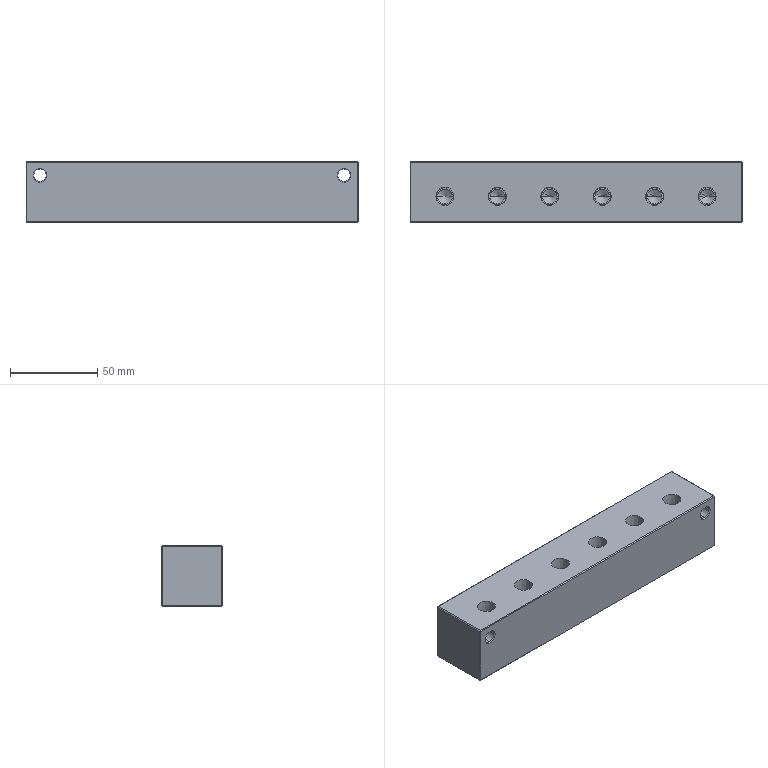Part | STEP file | OP10-011_junction block (B) | 1 solid | 122 faces | box 190 x 35 x 35 mm | volume 212721 mm3 | cone 44 | plane 40 | cylinder 38 | commonest cylinder face diameters 8.433 x30 7 x4 11 x4